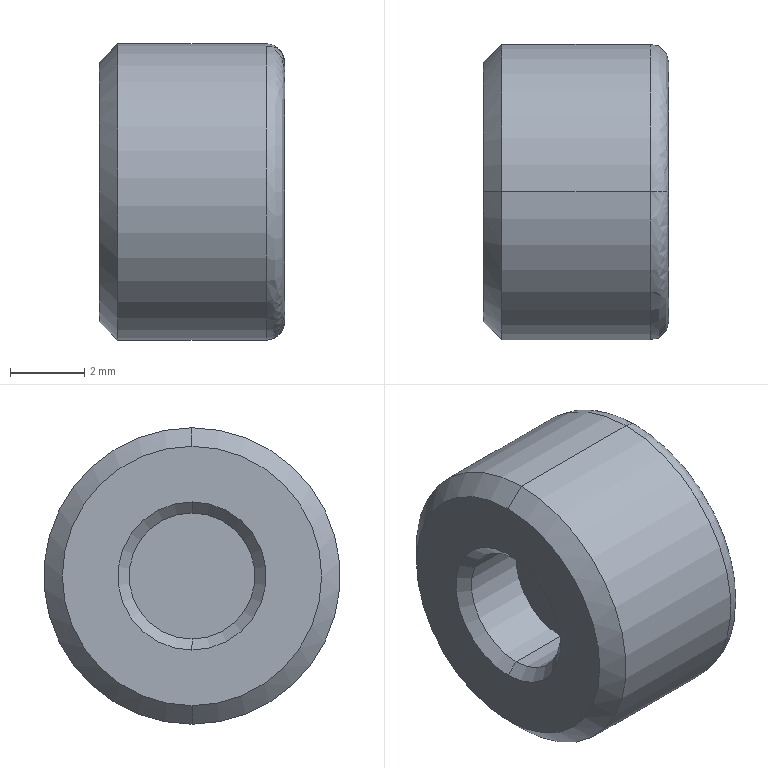Part | SolidWorks | features BaseBody 1 | 1 solid | 13 faces | box 5 x 8 x 8 mm | volume 228.346 mm3 | cylinder 4 | cone 4 | plane 3 | spline 2 | commonest cylinder face diameters 3.4 x2 8 x2
STEP:
#1=CARTESIAN_POINT('',(5.,0.,-3.5));
#2=VERTEX_POINT('',#1);
#3=CARTESIAN_POINT('',(5.,0.,3.5));
#4=VERTEX_POINT('',#3);
#5=CARTESIAN_POINT('',(5.,0.,-3.5));
#6=CARTESIAN_POINT('',(5.,-7.,-3.5));
#7=CARTESIAN_POINT('',(5.,-7.,3.5));
#8=CARTESIAN_POINT('',(5.,0.,3.5));
#9=(BOUNDED_CURVE()B_SPLINE_CURVE(3,(#5,#6,#7,#8),.UNSPECIFIED.,.F.,.F.)B_SPLINE_CURVE_WITH_KNOTS((4,4),(0.,1.),.UNSPECIFIED.)CURVE()GEOMETRIC_REPRESENTATION_ITEM()RATIONAL_B_SPLINE_CURVE((1.,0.3333,0.3333,1.))REPRESENTATION_ITEM(''));
#10=EDGE_CURVE('',#2,#4,#9,.T.);
#11=ORIENTED_EDGE('',*,*,#10,.T.);
#12=CARTESIAN_POINT('',(4.5,0.,4.));
#13=VERTEX_POINT('',#12);
#14=CARTESIAN_POINT('',(4.5,0.,3.5));
#15=DIRECTION('',(0.,-1.,0.));
#16=DIRECTION('',(0.,0.,1.));
#17=AXIS2_PLACEMENT_3D('',#14,#15,#16);
#18=CIRCLE('',#17,0.5);
#19=EDGE_CURVE('',#4,#13,#18,.T.);
#20=ORIENTED_EDGE('',*,*,#19,.T.);
#21=CARTESIAN_POINT('',(4.5,0.,-4.));
#22=VERTEX_POINT('',#21);
#23=CARTESIAN_POINT('',(4.5,0.,0.));
#24=DIRECTION('',(-1.,0.,0.));
#25=DIRECTION('',(0.,0.,-1.));
#26=AXIS2_PLACEMENT_3D('',#23,#24,#25);
#27=CIRCLE('',#26,4.);
#28=EDGE_CURVE('',#22,#13,#27,.T.);
#29=ORIENTED_EDGE('',*,*,#28,.F.);
#30=CARTESIAN_POINT('',(4.5,0.,-3.5));
#31=DIRECTION('',(0.,1.,0.));
#32=DIRECTION('',(0.,0.,-1.));
#33=AXIS2_PLACEMENT_3D('',#30,#31,#32);
#34=CIRCLE('',#33,0.5);
#35=EDGE_CURVE('',#2,#22,#34,.T.);
#36=ORIENTED_EDGE('',*,*,#35,.F.);
#37=EDGE_LOOP('',(#11,#20,#29,#36));
#38=FACE_OUTER_BOUND('',#37,.T.);
#39=CARTESIAN_POINT('',(5.,0.,3.5));
#40=CARTESIAN_POINT('',(5.,-7.,3.5));
#41=CARTESIAN_POINT('',(5.,-7.,-3.5));
#42=CARTESIAN_POINT('',(5.,0.,-3.5));
#43=CARTESIAN_POINT('',(5.,0.,3.793));
#44=CARTESIAN_POINT('',(5.,-7.586,3.793));
#45=CARTESIAN_POINT('',(5.,-7.586,-3.793));
#46=CARTESIAN_POINT('',(5.,0.,-3.793));
#47=CARTESIAN_POINT('',(4.793,0.,4.));
#48=CARTESIAN_POINT('',(4.793,-8.,4.));
#49=CARTESIAN_POINT('',(4.793,-8.,-4.));
#50=CARTESIAN_POINT('',(4.793,0.,-4.));
#51=CARTESIAN_POINT('',(4.5,0.,4.));
#52=CARTESIAN_POINT('',(4.5,-8.,4.));
#53=CARTESIAN_POINT('',(4.5,-8.,-4.));
#54=CARTESIAN_POINT('',(4.5,0.,-4.));
#55=(BOUNDED_SURFACE()B_SPLINE_SURFACE(3,3,((#39,#40,#41,#42),(#43,#44,#45,#46),(#47,#48,#49,#50),(#51,#52,#53,#54)),.UNSPECIFIED.,.F.,.F.,.F.)B_SPLINE_SURFACE_WITH_KNOTS((4,4),(4,4),(0.,1.),(0.,1.),.UNSPECIFIED.)GEOMETRIC_REPRESENTATION_ITEM()RATIONAL_B_SPLINE_SURFACE(((1.,0.3333,0.3333,1.),(0.8047,0.2682,0.2682,0.8047),(0.8047,0.2682,0.2682,0.8047),(1.,0.3333,0.3333,1.)))REPRESENTATION_ITEM('')SURFACE());
#56=ADVANCED_FACE('',(#38),#55,.T.);
#57=CARTESIAN_POINT('',(0.5,0.,-4.));
#58=VERTEX_POINT('',#57);
#59=CARTESIAN_POINT('',(0.5,0.,4.));
#60=VERTEX_POINT('',#59);
#61=CARTESIAN_POINT('',(0.5,0.,0.));
#62=DIRECTION('',(1.,0.,0.));
#63=DIRECTION('',(0.,0.,-1.));
#64=AXIS2_PLACEMENT_3D('',#61,#62,#63);
#65=CIRCLE('',#64,4.);
#66=EDGE_CURVE('',#58,#60,#65,.T.);
#67=ORIENTED_EDGE('',*,*,#66,.T.);
#68=CARTESIAN_POINT('',(0.,0.,4.));
#69=DIRECTION('',(1.,0.,0.));
#70=VECTOR('',#69,1000.);
#71=LINE('',#68,#70);
#72=EDGE_CURVE('',#60,#13,#71,.T.);
#73=ORIENTED_EDGE('',*,*,#72,.T.);
#74=CARTESIAN_POINT('',(4.5,0.,0.));
#75=DIRECTION('',(-1.,0.,0.));
#76=DIRECTION('',(0.,0.,-1.));
#77=AXIS2_PLACEMENT_3D('',#74,#75,#76);
#78=CIRCLE('',#77,4.);
#79=EDGE_CURVE('',#13,#22,#78,.T.);
#80=ORIENTED_EDGE('',*,*,#79,.T.);
#81=CARTESIAN_POINT('',(0.,0.,-4.));
#82=DIRECTION('',(1.,0.,0.));
#83=VECTOR('',#82,1000.);
#84=LINE('',#81,#83);
#85=EDGE_CURVE('',#58,#22,#84,.T.);
#86=ORIENTED_EDGE('',*,*,#85,.F.);
#87=EDGE_LOOP('',(#67,#73,#80,#86));
#88=FACE_OUTER_BOUND('',#87,.T.);
#89=CARTESIAN_POINT('',(0.,0.,0.));
#90=DIRECTION('',(1.,0.,0.));
#91=DIRECTION('',(0.,0.,-1.));
#92=AXIS2_PLACEMENT_3D('',#89,#90,#91);
#93=CYLINDRICAL_SURFACE('',#92,4.);
#94=ADVANCED_FACE('',(#88),#93,.T.);
#95=CARTESIAN_POINT('',(0.,0.,-3.5));
#96=VERTEX_POINT('',#95);
#97=CARTESIAN_POINT('',(0.,0.,3.5));
#98=VERTEX_POINT('',#97);
#99=CARTESIAN_POINT('',(0.,0.,0.));
#100=DIRECTION('',(1.,0.,0.));
#101=DIRECTION('',(0.,0.,-1.));
#102=AXIS2_PLACEMENT_3D('',#99,#100,#101);
#103=CIRCLE('',#102,3.5);
#104=EDGE_CURVE('',#96,#98,#103,.T.);
#105=ORIENTED_EDGE('',*,*,#104,.T.);
#106=CARTESIAN_POINT('',(0.5,0.,4.));
#107=DIRECTION('',(0.7071,0.,0.7071));
#108=VECTOR('',#107,1000.);
#109=LINE('',#106,#108);
#110=EDGE_CURVE('',#98,#60,#109,.T.);
#111=ORIENTED_EDGE('',*,*,#110,.T.);
#112=ORIENTED_EDGE('',*,*,#66,.F.);
#113=CARTESIAN_POINT('',(0.5,0.,-4.));
#114=DIRECTION('',(0.7071,0.,-0.7071));
#115=VECTOR('',#114,1000.);
#116=LINE('',#113,#115);
#117=EDGE_CURVE('',#96,#58,#116,.T.);
#118=ORIENTED_EDGE('',*,*,#117,.F.);
#119=EDGE_LOOP('',(#105,#111,#112,#118));
#120=FACE_OUTER_BOUND('',#119,.T.);
#121=CARTESIAN_POINT('',(0.5,0.,0.));
#122=DIRECTION('',(1.,0.,0.));
#123=DIRECTION('',(0.,0.,-1.));
#124=AXIS2_PLACEMENT_3D('',#121,#122,#123);
#125=CONICAL_SURFACE('',#124,4.,0.7854);
#126=ADVANCED_FACE('',(#120),#125,.T.);
#127=CARTESIAN_POINT('',(0.3,0.,-1.7));
#128=VERTEX_POINT('',#127);
#129=CARTESIAN_POINT('',(0.3,0.,1.7));
#130=VERTEX_POINT('',#129);
#131=CARTESIAN_POINT('',(0.3,0.,0.));
#132=DIRECTION('',(-1.,0.,0.));
#133=DIRECTION('',(0.,0.,1.));
#134=AXIS2_PLACEMENT_3D('',#131,#132,#133);
#135=CIRCLE('',#134,1.7);
#136=EDGE_CURVE('',#128,#130,#135,.T.);
#137=ORIENTED_EDGE('',*,*,#136,.F.);
#138=CARTESIAN_POINT('',(0.,0.,-2.));
#139=VERTEX_POINT('',#138);
#140=CARTESIAN_POINT('',(0.,0.,-2.));
#141=DIRECTION('',(-0.7071,0.,-0.7071));
#142=VECTOR('',#141,1000.);
#143=LINE('',#140,#142);
#144=EDGE_CURVE('',#128,#139,#143,.T.);
#145=ORIENTED_EDGE('',*,*,#144,.T.);
#146=CARTESIAN_POINT('',(0.,0.,2.));
#147=VERTEX_POINT('',#146);
#148=CARTESIAN_POINT('',(0.,0.,0.));
#149=DIRECTION('',(1.,0.,0.));
#150=DIRECTION('',(0.,0.,1.));
#151=AXIS2_PLACEMENT_3D('',#148,#149,#150);
#152=CIRCLE('',#151,2.);
#153=EDGE_CURVE('',#147,#139,#152,.T.);
#154=ORIENTED_EDGE('',*,*,#153,.F.);
#155=CARTESIAN_POINT('',(0.,0.,2.));
#156=DIRECTION('',(-0.7071,0.,0.7071));
#157=VECTOR('',#156,1000.);
#158=LINE('',#155,#157);
#159=EDGE_CURVE('',#130,#147,#158,.T.);
#160=ORIENTED_EDGE('',*,*,#159,.F.);
#161=EDGE_LOOP('',(#137,#145,#154,#160));
#162=FACE_OUTER_BOUND('',#161,.T.);
#163=CARTESIAN_POINT('',(0.,0.,0.));
#164=DIRECTION('',(-1.,0.,0.));
#165=DIRECTION('',(0.,0.,1.));
#166=AXIS2_PLACEMENT_3D('',#163,#164,#165);
#167=CONICAL_SURFACE('',#166,2.,0.7854);
#168=ADVANCED_FACE('',(#162),#167,.F.);
#169=CARTESIAN_POINT('',(2.,0.,-1.7));
#170=VERTEX_POINT('',#169);
#171=CARTESIAN_POINT('',(2.,0.,1.7));
#172=VERTEX_POINT('',#171);
#173=CARTESIAN_POINT('',(2.,0.,0.));
#174=DIRECTION('',(-1.,0.,0.));
#175=DIRECTION('',(0.,0.,1.));
#176=AXIS2_PLACEMENT_3D('',#173,#174,#175);
#177=CIRCLE('',#176,1.7);
#178=EDGE_CURVE('',#170,#172,#177,.T.);
#179=ORIENTED_EDGE('',*,*,#178,.F.);
#180=CARTESIAN_POINT('',(2.,0.,-1.7));
#181=DIRECTION('',(-1.,0.,0.));
#182=VECTOR('',#181,1000.);
#183=LINE('',#180,#182);
#184=EDGE_CURVE('',#170,#128,#183,.T.);
#185=ORIENTED_EDGE('',*,*,#184,.T.);
#186=ORIENTED_EDGE('',*,*,#136,.T.);
#187=CARTESIAN_POINT('',(2.,0.,1.7));
#188=DIRECTION('',(-1.,0.,0.));
#189=VECTOR('',#188,1000.);
#190=LINE('',#187,#189);
#191=EDGE_CURVE('',#172,#130,#190,.T.);
#192=ORIENTED_EDGE('',*,*,#191,.F.);
#193=EDGE_LOOP('',(#179,#185,#186,#192));
#194=FACE_OUTER_BOUND('',#193,.T.);
#195=CARTESIAN_POINT('',(2.,0.,0.));
#196=DIRECTION('',(-1.,0.,0.));
#197=DIRECTION('',(0.,0.,1.));
#198=AXIS2_PLACEMENT_3D('',#195,#196,#197);
#199=CYLINDRICAL_SURFACE('',#198,1.7);
#200=ADVANCED_FACE('',(#194),#199,.F.);
#201=ORIENTED_EDGE('',*,*,#72,.F.);
#202=CARTESIAN_POINT('',(0.5,0.,0.));
#203=DIRECTION('',(1.,0.,0.));
#204=DIRECTION('',(0.,0.,-1.));
#205=AXIS2_PLACEMENT_3D('',#202,#203,#204);
#206=CIRCLE('',#205,4.);
#207=EDGE_CURVE('',#60,#58,#206,.T.);
#208=ORIENTED_EDGE('',*,*,#207,.T.);
#209=ORIENTED_EDGE('',*,*,#85,.T.);
#210=ORIENTED_EDGE('',*,*,#28,.T.);
#211=EDGE_LOOP('',(#201,#208,#209,#210));
#212=FACE_OUTER_BOUND('',#211,.T.);
#213=CARTESIAN_POINT('',(0.,0.,0.));
#214=DIRECTION('',(1.,0.,0.));
#215=DIRECTION('',(0.,0.,-1.));
#216=AXIS2_PLACEMENT_3D('',#213,#214,#215);
#217=CYLINDRICAL_SURFACE('',#216,4.);
#218=ADVANCED_FACE('',(#212),#217,.T.);
#219=ORIENTED_EDGE('',*,*,#19,.F.);
#220=CARTESIAN_POINT('',(5.,0.,3.5));
#221=CARTESIAN_POINT('',(5.,7.,3.5));
#222=CARTESIAN_POINT('',(5.,7.,-3.5));
#223=CARTESIAN_POINT('',(5.,0.,-3.5));
#224=(BOUNDED_CURVE()B_SPLINE_CURVE(3,(#220,#221,#222,#223),.UNSPECIFIED.,.F.,.F.)B_SPLINE_CURVE_WITH_KNOTS((4,4),(0.,1.),.UNSPECIFIED.)CURVE()GEOMETRIC_REPRESENTATION_ITEM()RATIONAL_B_SPLINE_CURVE((1.,0.3333,0.3333,1.))REPRESENTATION_ITEM(''));
#225=EDGE_CURVE('',#4,#2,#224,.T.);
#226=ORIENTED_EDGE('',*,*,#225,.T.);
#227=ORIENTED_EDGE('',*,*,#35,.T.);
#228=ORIENTED_EDGE('',*,*,#79,.F.);
#229=EDGE_LOOP('',(#219,#226,#227,#228));
#230=FACE_OUTER_BOUND('',#229,.T.);
#231=CARTESIAN_POINT('',(5.,0.,-3.5));
#232=CARTESIAN_POINT('',(5.,7.,-3.5));
#233=CARTESIAN_POINT('',(5.,7.,3.5));
#234=CARTESIAN_POINT('',(5.,0.,3.5));
#235=CARTESIAN_POINT('',(5.,0.,-3.793));
#236=CARTESIAN_POINT('',(5.,7.586,-3.793));
#237=CARTESIAN_POINT('',(5.,7.586,3.793));
#238=CARTESIAN_POINT('',(5.,0.,3.793));
#239=CARTESIAN_POINT('',(4.793,0.,-4.));
#240=CARTESIAN_POINT('',(4.793,8.,-4.));
#241=CARTESIAN_POINT('',(4.793,8.,4.));
#242=CARTESIAN_POINT('',(4.793,0.,4.));
#243=CARTESIAN_POINT('',(4.5,0.,-4.));
#244=CARTESIAN_POINT('',(4.5,8.,-4.));
#245=CARTESIAN_POINT('',(4.5,8.,4.));
#246=CARTESIAN_POINT('',(4.5,0.,4.));
#247=(BOUNDED_SURFACE()B_SPLINE_SURFACE(3,3,((#231,#232,#233,#234),(#235,#236,#237,#238),(#239,#240,#241,#242),(#243,#244,#245,#246)),.UNSPECIFIED.,.F.,.F.,.F.)B_SPLINE_SURFACE_WITH_KNOTS((4,4),(4,4),(0.,1.),(0.,1.),.UNSPECIFIED.)GEOMETRIC_REPRESENTATION_ITEM()RATIONAL_B_SPLINE_SURFACE(((1.,0.3333,0.3333,1.),(0.8047,0.2682,0.2682,0.8047),(0.8047,0.2682,0.2682,0.8047),(1.,0.3333,0.3333,1.)))REPRESENTATION_ITEM('')SURFACE());
#248=ADVANCED_FACE('',(#230),#247,.T.);
#249=ORIENTED_EDGE('',*,*,#110,.F.);
#250=CARTESIAN_POINT('',(0.,0.,0.));
#251=DIRECTION('',(1.,0.,0.));
#252=DIRECTION('',(0.,0.,-1.));
#253=AXIS2_PLACEMENT_3D('',#250,#251,#252);
#254=CIRCLE('',#253,3.5);
#255=EDGE_CURVE('',#98,#96,#254,.T.);
#256=ORIENTED_EDGE('',*,*,#255,.T.);
#257=ORIENTED_EDGE('',*,*,#117,.T.);
#258=ORIENTED_EDGE('',*,*,#207,.F.);
#259=EDGE_LOOP('',(#249,#256,#257,#258));
#260=FACE_OUTER_BOUND('',#259,.T.);
#261=CARTESIAN_POINT('',(0.5,0.,0.));
#262=DIRECTION('',(1.,0.,0.));
#263=DIRECTION('',(0.,0.,-1.));
#264=AXIS2_PLACEMENT_3D('',#261,#262,#263);
#265=CONICAL_SURFACE('',#264,4.,0.7854);
#266=ADVANCED_FACE('',(#260),#265,.T.);
#267=ORIENTED_EDGE('',*,*,#225,.F.);
#268=ORIENTED_EDGE('',*,*,#10,.F.);
#269=EDGE_LOOP('',(#267,#268));
#270=FACE_OUTER_BOUND('',#269,.T.);
#271=CARTESIAN_POINT('',(5.,4.,0.));
#272=DIRECTION('',(1.,0.,0.));
#273=DIRECTION('',(0.,0.,-1.));
#274=AXIS2_PLACEMENT_3D('',#271,#272,#273);
#275=PLANE('',#274);
#276=ADVANCED_FACE('',(#270),#275,.T.);
#277=ORIENTED_EDGE('',*,*,#153,.T.);
#278=CARTESIAN_POINT('',(0.,0.,0.));
#279=DIRECTION('',(1.,0.,0.));
#280=DIRECTION('',(0.,0.,1.));
#281=AXIS2_PLACEMENT_3D('',#278,#279,#280);
#282=CIRCLE('',#281,2.);
#283=EDGE_CURVE('',#139,#147,#282,.T.);
#284=ORIENTED_EDGE('',*,*,#283,.T.);
#285=EDGE_LOOP('',(#277,#284));
#286=FACE_BOUND('',#285,.T.);
#287=ORIENTED_EDGE('',*,*,#104,.F.);
#288=ORIENTED_EDGE('',*,*,#255,.F.);
#289=EDGE_LOOP('',(#287,#288));
#290=FACE_OUTER_BOUND('',#289,.T.);
#291=CARTESIAN_POINT('',(0.,0.,0.));
#292=DIRECTION('',(-1.,0.,0.));
#293=DIRECTION('',(0.,0.,1.));
#294=AXIS2_PLACEMENT_3D('',#291,#292,#293);
#295=PLANE('',#294);
#296=ADVANCED_FACE('',(#286,#290),#295,.T.);
#297=ORIENTED_EDGE('',*,*,#144,.F.);
#298=CARTESIAN_POINT('',(0.3,0.,0.));
#299=DIRECTION('',(-1.,0.,0.));
#300=DIRECTION('',(0.,0.,1.));
#301=AXIS2_PLACEMENT_3D('',#298,#299,#300);
#302=CIRCLE('',#301,1.7);
#303=EDGE_CURVE('',#130,#128,#302,.T.);
#304=ORIENTED_EDGE('',*,*,#303,.F.);
#305=ORIENTED_EDGE('',*,*,#159,.T.);
#306=ORIENTED_EDGE('',*,*,#283,.F.);
#307=EDGE_LOOP('',(#297,#304,#305,#306));
#308=FACE_OUTER_BOUND('',#307,.T.);
#309=CARTESIAN_POINT('',(0.,0.,0.));
#310=DIRECTION('',(-1.,0.,0.));
#311=DIRECTION('',(0.,0.,1.));
#312=AXIS2_PLACEMENT_3D('',#309,#310,#311);
#313=CONICAL_SURFACE('',#312,2.,0.7854);
#314=ADVANCED_FACE('',(#308),#313,.F.);
#315=ORIENTED_EDGE('',*,*,#184,.F.);
#316=CARTESIAN_POINT('',(2.,0.,0.));
#317=DIRECTION('',(-1.,0.,0.));
#318=DIRECTION('',(0.,0.,1.));
#319=AXIS2_PLACEMENT_3D('',#316,#317,#318);
#320=CIRCLE('',#319,1.7);
#321=EDGE_CURVE('',#172,#170,#320,.T.);
#322=ORIENTED_EDGE('',*,*,#321,.F.);
#323=ORIENTED_EDGE('',*,*,#191,.T.);
#324=ORIENTED_EDGE('',*,*,#303,.T.);
#325=EDGE_LOOP('',(#315,#322,#323,#324));
#326=FACE_OUTER_BOUND('',#325,.T.);
#327=CARTESIAN_POINT('',(2.,0.,0.));
#328=DIRECTION('',(-1.,0.,0.));
#329=DIRECTION('',(0.,0.,1.));
#330=AXIS2_PLACEMENT_3D('',#327,#328,#329);
#331=CYLINDRICAL_SURFACE('',#330,1.7);
#332=ADVANCED_FACE('',(#326),#331,.F.);
#333=ORIENTED_EDGE('',*,*,#321,.T.);
#334=ORIENTED_EDGE('',*,*,#178,.T.);
#335=EDGE_LOOP('',(#333,#334));
#336=FACE_OUTER_BOUND('',#335,.T.);
#337=CARTESIAN_POINT('',(2.,0.,0.));
#338=DIRECTION('',(-1.,0.,0.));
#339=DIRECTION('',(0.,0.,1.));
#340=AXIS2_PLACEMENT_3D('',#337,#338,#339);
#341=PLANE('',#340);
#342=ADVANCED_FACE('',(#336),#341,.T.);
#343=CLOSED_SHELL('',(#56,#94,#126,#168,#200,#218,#248,#266,#276,#296,#314,#332,#342));
#344=MANIFOLD_SOLID_BREP('',#343);
#345=CARTESIAN_POINT('',(0.,0.,0.));
#346=DIRECTION('',(0.,0.,1.));
#347=DIRECTION('',(1.,0.,0.));
#348=AXIS2_PLACEMENT_3D('',#345,#346,#347);
#349=(LENGTH_UNIT()NAMED_UNIT(*)SI_UNIT(.MILLI.,.METRE.));
#350=UNCERTAINTY_MEASURE_WITH_UNIT(LENGTH_MEASURE(0.00001),#349,'','');
#351=(NAMED_UNIT(*)PLANE_ANGLE_UNIT()SI_UNIT($,.RADIAN.));
#352=(NAMED_UNIT(*)SI_UNIT($,.STERADIAN.)SOLID_ANGLE_UNIT());
#353=(GEOMETRIC_REPRESENTATION_CONTEXT(3)GLOBAL_UNCERTAINTY_ASSIGNED_CONTEXT((#350))GLOBAL_UNIT_ASSIGNED_CONTEXT((#349,#351,#352))REPRESENTATION_CONTEXT('',''));
#354=ADVANCED_BREP_SHAPE_REPRESENTATION('',(#344,#348),#353);